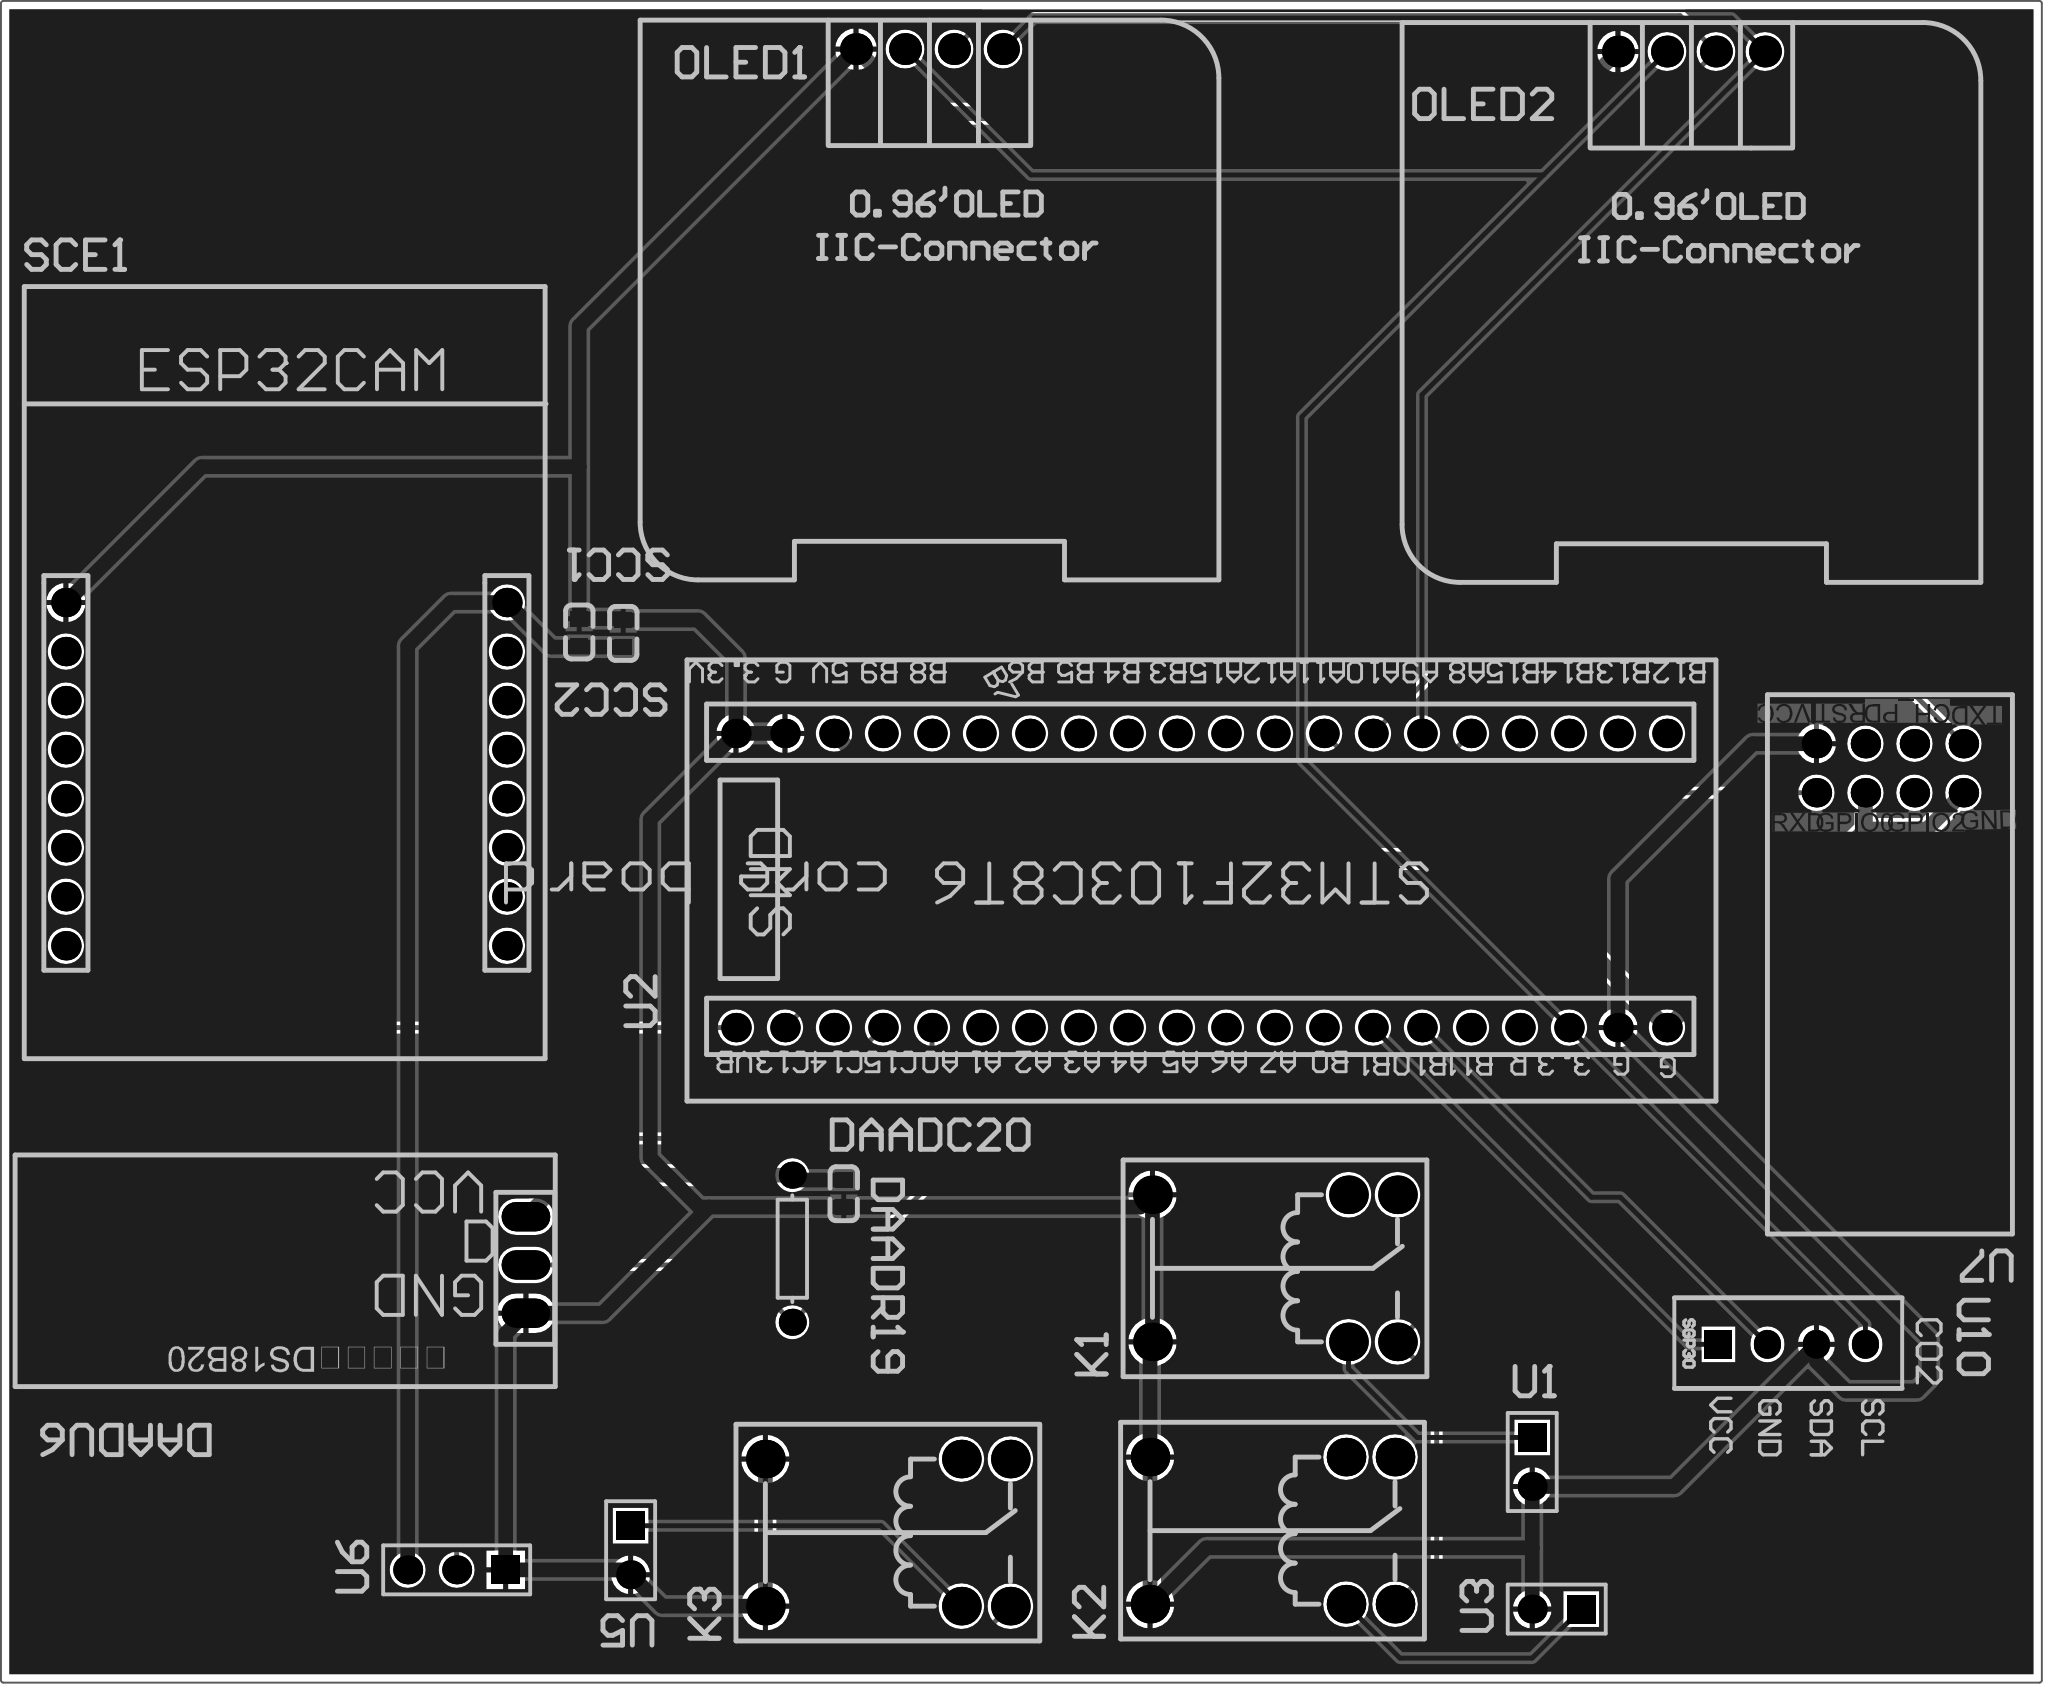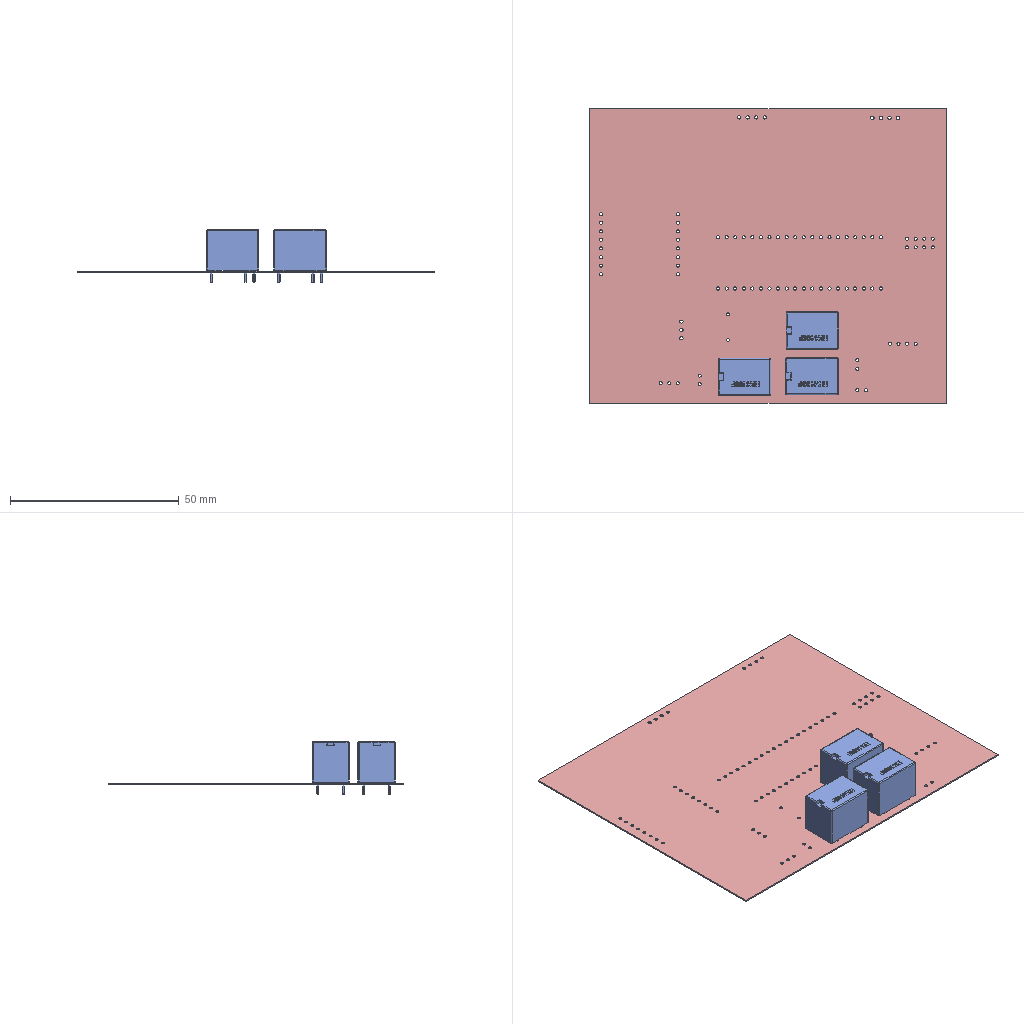Circuit board layout | Altium Designer | box 105.8 x 87.1 x 15.5 mm
Layer stack:
# Altium Designer layer stack of  (unit mm; dielectric type: 0 none, 1 core, 2 prepreg, 3 surface material)
index,name,kind,layer,copper_thickness_mm,dielectric_type,dielectric_thickness_mm,dielectric_material,dielectric_constant
0,Top Paste,other,,,,,,
1,Top Overlay,other,,,,,,
2,Top Solder,dielectric,,,3,0.0102,Solder Resist,3.5
3,Top Layer,copper,Top Layer,0.0356,,,,
4,Dielectric 1,dielectric,,,0,0.32,FR-4,4.8
5,Bottom Layer,copper,Bottom Layer,0.0356,,,,
6,Bottom Solder,dielectric,,,3,0.0102,Solder Resist,3.5
7,Bottom Overlay,other,,,,,,
8,Bottom Paste,other,,,,,,
# drill layer pairs: low layer,high layer
drill_pair,Top Layer,Bottom Layer
Part placement:
Designator,Comment,Layer,Footprint,Center-X(mm),Center-Y(mm),Rotation
U6,Turbidity module,TopLayer,HDR1X3,83.058,18.542,180
U10,SGP30,TopLayer,SGP30,152.273,30.226,270
U7,ESP-01S module,TopLayer,WIFI,157.353,60.071,270
U5,DC motor terminal,TopLayer,hdr1x2,92.075,19.558,270
U3,DC motor terminal,TopLayer,HDR1X2,140.081,16.51,180
U2,STM32F103C8T6 system board,TopLayer,STM32核心板,121.666,54.254,90
U1,DC motor terminal,TopLayer,HDR1X2,138.811,24.13,270
SCE1,ESP32CAM,TopLayer,ESP32CAM,74.231,59.764,0
SCC2,0.1u,TopLayer,C0603,89.408,67.121,270
SCC1,0.1uF,TopLayer,C0603,91.691,67.048,270
OLED2,0.96OLED_4P_MODULE_JX,TopLayer,0.96OLED_4P,147.065,97.2,360
OLED1,0.96OLED_4P_MODULE_JX,TopLayer,0.96OLED_4P,107.568,97.327,0
K3,HK4100F-DC3V-SHG relay,TopLayer,HK4100F,105.41,20.472,180
K2,HK4100F-DC3V-SHG relay,TopLayer,HK4100F,125.349,20.574,180
K1,HK4100F-DC3V-SHG relay,TopLayer,HK4100F,125.476,34.163,180
DAADU6,DS18B20+,TopLayer,DS18B20,86.648,34.338,180
DAADR19,4.7k,TopLayer,AXIAL-0.3,100.457,35.179,270
DAADC20,104,TopLayer,C0603,103.124,38.038,90
Pad and via stacks:
# Altium Designer via and pad stacks of  (unit mm). Each distinct definition once, with the count of objects using it.
# via: kind,start_layer,end_layer,hole_mm,diameter_mm,mode(0 simple;1 top-mid-bottom;2 full stack),diameter_per_layer,count,example_net
# pad: kind,layer,hole_mm,hole_type(0 round;1 square;2 slot),plating,top_size,top_shape(1 round;2 rect;3 octagon;9 rounded rect),mid_size,bottom_size,mode,footprint,size_per_layer,count,example
pad,Top Layer,0,0,plated,0.8x0.9,2,0.8x0.9,0.8x0.9,0,C0603,,6,SCC2.1
pad,Multi-Layer,0.9,0,plated,1.5x1.5,2,1.5x1.5,1.5x1.5,0,HDR1X3,,1,U6.1
pad,Multi-Layer,0.9,0,plated,1.5x1.5,1,1.5x1.5,1.5x1.5,0,HDR1X3,,2,U6.2
pad,Multi-Layer,0.9144,2,plated,1.524x1.524,1,1.524x1.524,1.524x1.524,0,STM32\u00BA\u00CB\u00D0\u00C4\u00B0\u00E5,,40,U2.1
pad,Multi-Layer,1,2,plated,1.65x1.65,1,1.65x1.65,1.65x1.65,0,0.96OLED_4P,,8,OLED1.4
pad,Multi-Layer,0.9,2,plated,1.4x1.5,1,1.4x1.5,1.4x1.5,0,SGP30,,3,U10.3
pad,Multi-Layer,0.9,2,plated,1.4x1.5,2,1.4x1.5,1.4x1.5,0,SGP30,,1,U10.1
pad,Multi-Layer,1,0,plated,2x2,1,2x2,2x2,0,HK4100F,,18,K3.3
pad,Multi-Layer,0.9,0,plated,1.524x1.524,1,1.524x1.524,1.524x1.524,0,ESP32CAM,,16,SCE1.9
pad,Multi-Layer,0.9,0,plated,1.5x1.5,2,1.5x1.5,1.5x1.5,0,hdr1x2,,3,U5.1
pad,Multi-Layer,0.9,0,plated,1.5x1.5,1,1.5x1.5,1.5x1.5,0,hdr1x2,,3,U5.2
pad,Multi-Layer,0.9144,0,plated,1.524x1.524,1,1.524x1.524,1.524x1.524,0,WIFI,,8,U7.8
pad,Multi-Layer,0.9,2,plated,2.524x1.524,1,2.524x1.524,2.524x1.524,0,DS18B20,,3,DAADU6.2
pad,Multi-Layer,0.85,0,plated,1.4x1.4,1,1.4x1.4,1.4x1.4,0,AXIAL-0.3,,2,DAADR19.2
Copper pours:
name,layer,net,type(0 solid;1 hatched;2 none)
Top Layer-No Net,Bottom Layer,GND,0
Top Layer-No Net,Top Layer,GND,0
Design rules, without the lines most boards share:
# Altium Designer design rules of  (exported by Altium Designer, unit mm)
# columns: name | kind | enabled | priority | scope1 | scope2 | descriptor | typed fields (field=value)
SilkToSilkClearance | 55 | enabled | 1 | All | All | Silk to Silk (Clearance=0mil) (All),(All) |
SilkToSolderMaskClearance | 54 | enabled | 1 | IsPad | All | Silk To Solder Mask (Clearance=0mil) (IsPad),(All) |
MinimumSolderMaskSliver | 53 | enabled | 1 | All | All | Minimum Solder Mask Sliver (Gap=0mil) (All),(All) |
HoleToHoleClearance | 52 | enabled | 1 | All | All | Hole To Hole Clearance (Gap=10mil) (All),(All) | gap=0.254
DiffPairsRouting | 51 | enabled | 1 | All | All | Differential Pairs Uncoupled Length using the Gap Constraints (Min=10mil) (Max=10mil) (Prefered=10mil)  and Width Constraints (Min=15mil) (Max=15mil) (Prefered=15mil) (All) |
SolderMaskExpansion | 13 | enabled | 1 | All | All | Solder Mask Expansion (Expansion =4mil) (All) | expansion=0.1016
PasteMaskExpansion | 14 | enabled | 1 | All | All | Paste Mask Expansion (Expansion =0mil) (All) | expansion=0
RoutingVias | 11 | enabled | 1 | All | All | Routing Via (MinHoleWidth=28mil) (MaxHoleWidth=28mil) (PreferredHoleWidth=28mil) (MinWidth=50mil) (MaxWidth=50mil) (PreferedWidth=50mil) (All) | via_min_hole=0.7112 via_max_hole=0.7112 via_preferred_diameter=1.27 via_preferred_hole=0.7112
Width | 2 | enabled | 1 | All | All | Width Constraint (Min=10mil) (Max=30mil) (Preferred=10mil) (All) |
PolygonConnect | 20 | enabled | 1 | All | All | Polygon Connect Rule(Relief Connect )(Conductor Width=10mil) (Relief Angle=90 Angle) (Entries=4) (Air Gap Width=10mil) (All),(All) | connect_style(0=relief,1=direct,2=none)=0 relief_conductor_width=0.254 relief_entries=4
PlaneConnect | 6 | enabled | 1 | All | All | Power Plane Connect Rule(Relief Connect )(Expansion=20mil) (Conductor Width=10mil) (Air Gap=10mil) (Entries=4) (All) | relief_conductor_width=0.254 relief_entries=4 relief_expansion=0.508
Clearance | 0 | enabled | 1 | All | All | Clearance Constraint (Gap=7mil) (All),(All) | gap=0.1778